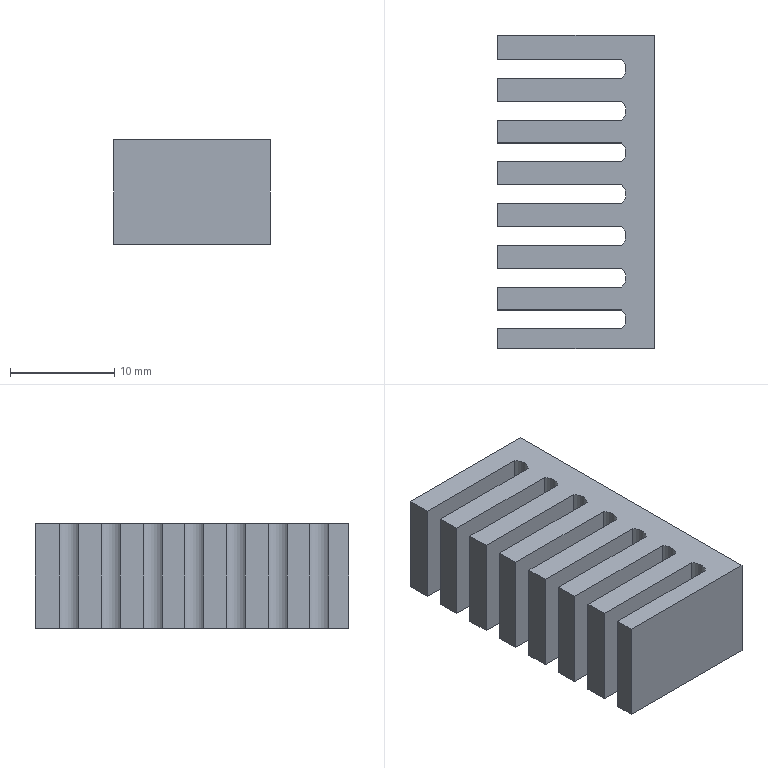Part | SolidWorks | features Extrusion 1 | 1 solid | 34 faces | box 15 x 30 x 10 mm | volume 2949 mm3 | plane 27 | cylinder 7 | commonest cylinder face diameters 2.576 x7
STEP:
#1=CARTESIAN_POINT('',(7.5,-15.,-5.));
#2=VERTEX_POINT('',#1);
#3=CARTESIAN_POINT('',(7.5,15.,-5.));
#4=VERTEX_POINT('',#3);
#5=CARTESIAN_POINT('',(7.5,-15.,-5.));
#6=DIRECTION('',(0.,1.,0.));
#7=VECTOR('',#6,1000.);
#8=LINE('',#5,#7);
#9=EDGE_CURVE('',#2,#4,#8,.T.);
#10=ORIENTED_EDGE('',*,*,#9,.T.);
#11=CARTESIAN_POINT('',(7.5,15.,5.));
#12=VERTEX_POINT('',#11);
#13=CARTESIAN_POINT('',(7.5,15.,5.));
#14=DIRECTION('',(0.,0.,-1.));
#15=VECTOR('',#14,1000.);
#16=LINE('',#13,#15);
#17=EDGE_CURVE('',#12,#4,#16,.T.);
#18=ORIENTED_EDGE('',*,*,#17,.F.);
#19=CARTESIAN_POINT('',(7.5,-15.,5.));
#20=VERTEX_POINT('',#19);
#21=CARTESIAN_POINT('',(7.5,-15.,5.));
#22=DIRECTION('',(0.,1.,0.));
#23=VECTOR('',#22,1000.);
#24=LINE('',#21,#23);
#25=EDGE_CURVE('',#20,#12,#24,.T.);
#26=ORIENTED_EDGE('',*,*,#25,.F.);
#27=CARTESIAN_POINT('',(7.5,-15.,5.));
#28=DIRECTION('',(0.,0.,-1.));
#29=VECTOR('',#28,1000.);
#30=LINE('',#27,#29);
#31=EDGE_CURVE('',#20,#2,#30,.T.);
#32=ORIENTED_EDGE('',*,*,#31,.T.);
#33=EDGE_LOOP('',(#10,#18,#26,#32));
#34=FACE_OUTER_BOUND('',#33,.T.);
#35=CARTESIAN_POINT('',(7.5,-15.,5.));
#36=DIRECTION('',(-1.,0.,0.));
#37=DIRECTION('',(0.,0.,1.));
#38=AXIS2_PLACEMENT_3D('',#35,#36,#37);
#39=PLANE('',#38);
#40=ADVANCED_FACE('',(#34),#39,.F.);
#41=CARTESIAN_POINT('',(-7.5,15.,-5.));
#42=VERTEX_POINT('',#41);
#43=CARTESIAN_POINT('',(7.5,15.,-5.));
#44=DIRECTION('',(-1.,0.,0.));
#45=VECTOR('',#44,1000.);
#46=LINE('',#43,#45);
#47=EDGE_CURVE('',#4,#42,#46,.T.);
#48=ORIENTED_EDGE('',*,*,#47,.T.);
#49=CARTESIAN_POINT('',(-7.5,15.,5.));
#50=VERTEX_POINT('',#49);
#51=CARTESIAN_POINT('',(-7.5,15.,5.));
#52=DIRECTION('',(0.,0.,-1.));
#53=VECTOR('',#52,1000.);
#54=LINE('',#51,#53);
#55=EDGE_CURVE('',#50,#42,#54,.T.);
#56=ORIENTED_EDGE('',*,*,#55,.F.);
#57=CARTESIAN_POINT('',(7.5,15.,5.));
#58=DIRECTION('',(-1.,0.,0.));
#59=VECTOR('',#58,1000.);
#60=LINE('',#57,#59);
#61=EDGE_CURVE('',#12,#50,#60,.T.);
#62=ORIENTED_EDGE('',*,*,#61,.F.);
#63=ORIENTED_EDGE('',*,*,#17,.T.);
#64=EDGE_LOOP('',(#48,#56,#62,#63));
#65=FACE_OUTER_BOUND('',#64,.T.);
#66=CARTESIAN_POINT('',(7.5,15.,5.));
#67=DIRECTION('',(0.,-1.,0.));
#68=DIRECTION('',(1.,0.,0.));
#69=AXIS2_PLACEMENT_3D('',#66,#67,#68);
#70=PLANE('',#69);
#71=ADVANCED_FACE('',(#65),#70,.F.);
#72=CARTESIAN_POINT('',(-7.5,12.696,-5.));
#73=VERTEX_POINT('',#72);
#74=CARTESIAN_POINT('',(-7.5,12.696,-5.));
#75=DIRECTION('',(0.,-1.,0.));
#76=VECTOR('',#75,1000.);
#77=LINE('',#74,#76);
#78=EDGE_CURVE('',#42,#73,#77,.T.);
#79=ORIENTED_EDGE('',*,*,#78,.T.);
#80=CARTESIAN_POINT('',(-7.5,12.696,5.));
#81=VERTEX_POINT('',#80);
#82=CARTESIAN_POINT('',(-7.5,12.696,5.));
#83=DIRECTION('',(0.,0.,-1.));
#84=VECTOR('',#83,1000.);
#85=LINE('',#82,#84);
#86=EDGE_CURVE('',#81,#73,#85,.T.);
#87=ORIENTED_EDGE('',*,*,#86,.F.);
#88=CARTESIAN_POINT('',(-7.5,12.696,5.));
#89=DIRECTION('',(0.,-1.,0.));
#90=VECTOR('',#89,1000.);
#91=LINE('',#88,#90);
#92=EDGE_CURVE('',#50,#81,#91,.T.);
#93=ORIENTED_EDGE('',*,*,#92,.F.);
#94=ORIENTED_EDGE('',*,*,#55,.T.);
#95=EDGE_LOOP('',(#79,#87,#93,#94));
#96=FACE_OUTER_BOUND('',#95,.T.);
#97=CARTESIAN_POINT('',(-7.5,12.696,5.));
#98=DIRECTION('',(1.,0.,0.));
#99=DIRECTION('',(0.,0.,-1.));
#100=AXIS2_PLACEMENT_3D('',#97,#98,#99);
#101=PLANE('',#100);
#102=ADVANCED_FACE('',(#96),#101,.F.);
#103=CARTESIAN_POINT('',(4.407,12.696,-5.));
#104=VERTEX_POINT('',#103);
#105=CARTESIAN_POINT('',(4.407,12.696,-5.));
#106=DIRECTION('',(1.,0.,0.));
#107=VECTOR('',#106,1000.);
#108=LINE('',#105,#107);
#109=EDGE_CURVE('',#73,#104,#108,.T.);
#110=ORIENTED_EDGE('',*,*,#109,.T.);
#111=CARTESIAN_POINT('',(4.407,12.696,5.));
#112=VERTEX_POINT('',#111);
#113=CARTESIAN_POINT('',(4.407,12.696,5.));
#114=DIRECTION('',(0.,0.,-1.));
#115=VECTOR('',#114,1000.);
#116=LINE('',#113,#115);
#117=EDGE_CURVE('',#112,#104,#116,.T.);
#118=ORIENTED_EDGE('',*,*,#117,.F.);
#119=CARTESIAN_POINT('',(4.407,12.696,5.));
#120=DIRECTION('',(1.,0.,0.));
#121=VECTOR('',#120,1000.);
#122=LINE('',#119,#121);
#123=EDGE_CURVE('',#81,#112,#122,.T.);
#124=ORIENTED_EDGE('',*,*,#123,.F.);
#125=ORIENTED_EDGE('',*,*,#86,.T.);
#126=EDGE_LOOP('',(#110,#118,#124,#125));
#127=FACE_OUTER_BOUND('',#126,.T.);
#128=CARTESIAN_POINT('',(4.407,12.696,5.));
#129=DIRECTION('',(0.,1.,0.));
#130=DIRECTION('',(0.,0.,1.));
#131=AXIS2_PLACEMENT_3D('',#128,#129,#130);
#132=PLANE('',#131);
#133=ADVANCED_FACE('',(#127),#132,.F.);
#134=CARTESIAN_POINT('',(4.407,10.874,-5.));
#135=VERTEX_POINT('',#134);
#136=CARTESIAN_POINT('',(3.497,11.785,-5.));
#137=DIRECTION('',(0.,0.,-1.));
#138=DIRECTION('',(1.,0.,0.));
#139=AXIS2_PLACEMENT_3D('',#136,#137,#138);
#140=CIRCLE('',#139,1.288);
#141=EDGE_CURVE('',#104,#135,#140,.T.);
#142=ORIENTED_EDGE('',*,*,#141,.T.);
#143=CARTESIAN_POINT('',(4.407,10.874,5.));
#144=VERTEX_POINT('',#143);
#145=CARTESIAN_POINT('',(4.407,10.874,5.));
#146=DIRECTION('',(0.,0.,-1.));
#147=VECTOR('',#146,1000.);
#148=LINE('',#145,#147);
#149=EDGE_CURVE('',#144,#135,#148,.T.);
#150=ORIENTED_EDGE('',*,*,#149,.F.);
#151=CARTESIAN_POINT('',(3.497,11.785,5.));
#152=DIRECTION('',(0.,0.,-1.));
#153=DIRECTION('',(1.,0.,0.));
#154=AXIS2_PLACEMENT_3D('',#151,#152,#153);
#155=CIRCLE('',#154,1.288);
#156=EDGE_CURVE('',#112,#144,#155,.T.);
#157=ORIENTED_EDGE('',*,*,#156,.F.);
#158=ORIENTED_EDGE('',*,*,#117,.T.);
#159=EDGE_LOOP('',(#142,#150,#157,#158));
#160=FACE_OUTER_BOUND('',#159,.T.);
#161=CARTESIAN_POINT('',(3.497,11.785,5.));
#162=DIRECTION('',(0.,0.,-1.));
#163=DIRECTION('',(-1.,0.,0.));
#164=AXIS2_PLACEMENT_3D('',#161,#162,#163);
#165=CYLINDRICAL_SURFACE('',#164,1.288);
#166=ADVANCED_FACE('',(#160),#165,.F.);
#167=CARTESIAN_POINT('',(-7.5,10.874,-5.));
#168=VERTEX_POINT('',#167);
#169=CARTESIAN_POINT('',(-7.5,10.874,-5.));
#170=DIRECTION('',(-1.,0.,0.));
#171=VECTOR('',#170,1000.);
#172=LINE('',#169,#171);
#173=EDGE_CURVE('',#135,#168,#172,.T.);
#174=ORIENTED_EDGE('',*,*,#173,.T.);
#175=CARTESIAN_POINT('',(-7.5,10.874,5.));
#176=VERTEX_POINT('',#175);
#177=CARTESIAN_POINT('',(-7.5,10.874,5.));
#178=DIRECTION('',(0.,0.,-1.));
#179=VECTOR('',#178,1000.);
#180=LINE('',#177,#179);
#181=EDGE_CURVE('',#176,#168,#180,.T.);
#182=ORIENTED_EDGE('',*,*,#181,.F.);
#183=CARTESIAN_POINT('',(-7.5,10.874,5.));
#184=DIRECTION('',(-1.,0.,0.));
#185=VECTOR('',#184,1000.);
#186=LINE('',#183,#185);
#187=EDGE_CURVE('',#144,#176,#186,.T.);
#188=ORIENTED_EDGE('',*,*,#187,.F.);
#189=ORIENTED_EDGE('',*,*,#149,.T.);
#190=EDGE_LOOP('',(#174,#182,#188,#189));
#191=FACE_OUTER_BOUND('',#190,.T.);
#192=CARTESIAN_POINT('',(-7.5,10.874,5.));
#193=DIRECTION('',(0.,-1.,0.));
#194=DIRECTION('',(0.,0.,-1.));
#195=AXIS2_PLACEMENT_3D('',#192,#193,#194);
#196=PLANE('',#195);
#197=ADVANCED_FACE('',(#191),#196,.F.);
#198=CARTESIAN_POINT('',(-7.5,8.696,-5.));
#199=VERTEX_POINT('',#198);
#200=CARTESIAN_POINT('',(-7.5,8.696,-5.));
#201=DIRECTION('',(0.,-1.,0.));
#202=VECTOR('',#201,1000.);
#203=LINE('',#200,#202);
#204=EDGE_CURVE('',#168,#199,#203,.T.);
#205=ORIENTED_EDGE('',*,*,#204,.T.);
#206=CARTESIAN_POINT('',(-7.5,8.696,5.));
#207=VERTEX_POINT('',#206);
#208=CARTESIAN_POINT('',(-7.5,8.696,5.));
#209=DIRECTION('',(0.,0.,-1.));
#210=VECTOR('',#209,1000.);
#211=LINE('',#208,#210);
#212=EDGE_CURVE('',#207,#199,#211,.T.);
#213=ORIENTED_EDGE('',*,*,#212,.F.);
#214=CARTESIAN_POINT('',(-7.5,8.696,5.));
#215=DIRECTION('',(0.,-1.,0.));
#216=VECTOR('',#215,1000.);
#217=LINE('',#214,#216);
#218=EDGE_CURVE('',#176,#207,#217,.T.);
#219=ORIENTED_EDGE('',*,*,#218,.F.);
#220=ORIENTED_EDGE('',*,*,#181,.T.);
#221=EDGE_LOOP('',(#205,#213,#219,#220));
#222=FACE_OUTER_BOUND('',#221,.T.);
#223=CARTESIAN_POINT('',(-7.5,8.696,5.));
#224=DIRECTION('',(1.,0.,0.));
#225=DIRECTION('',(0.,0.,-1.));
#226=AXIS2_PLACEMENT_3D('',#223,#224,#225);
#227=PLANE('',#226);
#228=ADVANCED_FACE('',(#222),#227,.F.);
#229=CARTESIAN_POINT('',(4.407,8.696,-5.));
#230=VERTEX_POINT('',#229);
#231=CARTESIAN_POINT('',(4.407,8.696,-5.));
#232=DIRECTION('',(1.,0.,0.));
#233=VECTOR('',#232,1000.);
#234=LINE('',#231,#233);
#235=EDGE_CURVE('',#199,#230,#234,.T.);
#236=ORIENTED_EDGE('',*,*,#235,.T.);
#237=CARTESIAN_POINT('',(4.407,8.696,5.));
#238=VERTEX_POINT('',#237);
#239=CARTESIAN_POINT('',(4.407,8.696,5.));
#240=DIRECTION('',(0.,0.,-1.));
#241=VECTOR('',#240,1000.);
#242=LINE('',#239,#241);
#243=EDGE_CURVE('',#238,#230,#242,.T.);
#244=ORIENTED_EDGE('',*,*,#243,.F.);
#245=CARTESIAN_POINT('',(4.407,8.696,5.));
#246=DIRECTION('',(1.,0.,0.));
#247=VECTOR('',#246,1000.);
#248=LINE('',#245,#247);
#249=EDGE_CURVE('',#207,#238,#248,.T.);
#250=ORIENTED_EDGE('',*,*,#249,.F.);
#251=ORIENTED_EDGE('',*,*,#212,.T.);
#252=EDGE_LOOP('',(#236,#244,#250,#251));
#253=FACE_OUTER_BOUND('',#252,.T.);
#254=CARTESIAN_POINT('',(4.407,8.696,5.));
#255=DIRECTION('',(0.,1.,0.));
#256=DIRECTION('',(0.,0.,1.));
#257=AXIS2_PLACEMENT_3D('',#254,#255,#256);
#258=PLANE('',#257);
#259=ADVANCED_FACE('',(#253),#258,.F.);
#260=CARTESIAN_POINT('',(4.407,6.874,-5.));
#261=VERTEX_POINT('',#260);
#262=CARTESIAN_POINT('',(3.497,7.785,-5.));
#263=DIRECTION('',(0.,0.,-1.));
#264=DIRECTION('',(1.,0.,0.));
#265=AXIS2_PLACEMENT_3D('',#262,#263,#264);
#266=CIRCLE('',#265,1.288);
#267=EDGE_CURVE('',#230,#261,#266,.T.);
#268=ORIENTED_EDGE('',*,*,#267,.T.);
#269=CARTESIAN_POINT('',(4.407,6.874,5.));
#270=VERTEX_POINT('',#269);
#271=CARTESIAN_POINT('',(4.407,6.874,5.));
#272=DIRECTION('',(0.,0.,-1.));
#273=VECTOR('',#272,1000.);
#274=LINE('',#271,#273);
#275=EDGE_CURVE('',#270,#261,#274,.T.);
#276=ORIENTED_EDGE('',*,*,#275,.F.);
#277=CARTESIAN_POINT('',(3.497,7.785,5.));
#278=DIRECTION('',(0.,0.,-1.));
#279=DIRECTION('',(1.,0.,0.));
#280=AXIS2_PLACEMENT_3D('',#277,#278,#279);
#281=CIRCLE('',#280,1.288);
#282=EDGE_CURVE('',#238,#270,#281,.T.);
#283=ORIENTED_EDGE('',*,*,#282,.F.);
#284=ORIENTED_EDGE('',*,*,#243,.T.);
#285=EDGE_LOOP('',(#268,#276,#283,#284));
#286=FACE_OUTER_BOUND('',#285,.T.);
#287=CARTESIAN_POINT('',(3.497,7.785,5.));
#288=DIRECTION('',(0.,0.,-1.));
#289=DIRECTION('',(-1.,0.,0.));
#290=AXIS2_PLACEMENT_3D('',#287,#288,#289);
#291=CYLINDRICAL_SURFACE('',#290,1.288);
#292=ADVANCED_FACE('',(#286),#291,.F.);
#293=CARTESIAN_POINT('',(-7.5,6.874,-5.));
#294=VERTEX_POINT('',#293);
#295=CARTESIAN_POINT('',(-7.5,6.874,-5.));
#296=DIRECTION('',(-1.,0.,0.));
#297=VECTOR('',#296,1000.);
#298=LINE('',#295,#297);
#299=EDGE_CURVE('',#261,#294,#298,.T.);
#300=ORIENTED_EDGE('',*,*,#299,.T.);
#301=CARTESIAN_POINT('',(-7.5,6.874,5.));
#302=VERTEX_POINT('',#301);
#303=CARTESIAN_POINT('',(-7.5,6.874,5.));
#304=DIRECTION('',(0.,0.,-1.));
#305=VECTOR('',#304,1000.);
#306=LINE('',#303,#305);
#307=EDGE_CURVE('',#302,#294,#306,.T.);
#308=ORIENTED_EDGE('',*,*,#307,.F.);
#309=CARTESIAN_POINT('',(-7.5,6.874,5.));
#310=DIRECTION('',(-1.,0.,0.));
#311=VECTOR('',#310,1000.);
#312=LINE('',#309,#311);
#313=EDGE_CURVE('',#270,#302,#312,.T.);
#314=ORIENTED_EDGE('',*,*,#313,.F.);
#315=ORIENTED_EDGE('',*,*,#275,.T.);
#316=EDGE_LOOP('',(#300,#308,#314,#315));
#317=FACE_OUTER_BOUND('',#316,.T.);
#318=CARTESIAN_POINT('',(-7.5,6.874,5.));
#319=DIRECTION('',(0.,-1.,0.));
#320=DIRECTION('',(0.,0.,-1.));
#321=AXIS2_PLACEMENT_3D('',#318,#319,#320);
#322=PLANE('',#321);
#323=ADVANCED_FACE('',(#317),#322,.F.);
#324=CARTESIAN_POINT('',(-7.5,4.696,-5.));
#325=VERTEX_POINT('',#324);
#326=CARTESIAN_POINT('',(-7.5,6.874,-5.));
#327=DIRECTION('',(0.,-1.,0.));
#328=VECTOR('',#327,1000.);
#329=LINE('',#326,#328);
#330=EDGE_CURVE('',#294,#325,#329,.T.);
#331=ORIENTED_EDGE('',*,*,#330,.T.);
#332=CARTESIAN_POINT('',(-7.5,4.696,5.));
#333=VERTEX_POINT('',#332);
#334=CARTESIAN_POINT('',(-7.5,4.696,5.));
#335=DIRECTION('',(0.,0.,-1.));
#336=VECTOR('',#335,1000.);
#337=LINE('',#334,#336);
#338=EDGE_CURVE('',#333,#325,#337,.T.);
#339=ORIENTED_EDGE('',*,*,#338,.F.);
#340=CARTESIAN_POINT('',(-7.5,6.874,5.));
#341=DIRECTION('',(0.,-1.,0.));
#342=VECTOR('',#341,1000.);
#343=LINE('',#340,#342);
#344=EDGE_CURVE('',#302,#333,#343,.T.);
#345=ORIENTED_EDGE('',*,*,#344,.F.);
#346=ORIENTED_EDGE('',*,*,#307,.T.);
#347=EDGE_LOOP('',(#331,#339,#345,#346));
#348=FACE_OUTER_BOUND('',#347,.T.);
#349=CARTESIAN_POINT('',(-7.5,6.874,5.));
#350=DIRECTION('',(1.,0.,0.));
#351=DIRECTION('',(0.,0.,-1.));
#352=AXIS2_PLACEMENT_3D('',#349,#350,#351);
#353=PLANE('',#352);
#354=ADVANCED_FACE('',(#348),#353,.F.);
#355=CARTESIAN_POINT('',(4.407,4.696,-5.));
#356=VERTEX_POINT('',#355);
#357=CARTESIAN_POINT('',(4.407,4.696,-5.));
#358=DIRECTION('',(1.,0.,0.));
#359=VECTOR('',#358,1000.);
#360=LINE('',#357,#359);
#361=EDGE_CURVE('',#325,#356,#360,.T.);
#362=ORIENTED_EDGE('',*,*,#361,.T.);
#363=CARTESIAN_POINT('',(4.407,4.696,5.));
#364=VERTEX_POINT('',#363);
#365=CARTESIAN_POINT('',(4.407,4.696,5.));
#366=DIRECTION('',(0.,0.,-1.));
#367=VECTOR('',#366,1000.);
#368=LINE('',#365,#367);
#369=EDGE_CURVE('',#364,#356,#368,.T.);
#370=ORIENTED_EDGE('',*,*,#369,.F.);
#371=CARTESIAN_POINT('',(4.407,4.696,5.));
#372=DIRECTION('',(1.,0.,0.));
#373=VECTOR('',#372,1000.);
#374=LINE('',#371,#373);
#375=EDGE_CURVE('',#333,#364,#374,.T.);
#376=ORIENTED_EDGE('',*,*,#375,.F.);
#377=ORIENTED_EDGE('',*,*,#338,.T.);
#378=EDGE_LOOP('',(#362,#370,#376,#377));
#379=FACE_OUTER_BOUND('',#378,.T.);
#380=CARTESIAN_POINT('',(4.407,4.696,5.));
#381=DIRECTION('',(0.,1.,0.));
#382=DIRECTION('',(0.,0.,1.));
#383=AXIS2_PLACEMENT_3D('',#380,#381,#382);
#384=PLANE('',#383);
#385=ADVANCED_FACE('',(#379),#384,.F.);
#386=CARTESIAN_POINT('',(4.407,2.874,-5.));
#387=VERTEX_POINT('',#386);
#388=CARTESIAN_POINT('',(3.497,3.785,-5.));
#389=DIRECTION('',(0.,0.,-1.));
#390=DIRECTION('',(1.,0.,0.));
#391=AXIS2_PLACEMENT_3D('',#388,#389,#390);
#392=CIRCLE('',#391,1.288);
#393=EDGE_CURVE('',#356,#387,#392,.T.);
#394=ORIENTED_EDGE('',*,*,#393,.T.);
#395=CARTESIAN_POINT('',(4.407,2.874,5.));
#396=VERTEX_POINT('',#395);
#397=CARTESIAN_POINT('',(4.407,2.874,5.));
#398=DIRECTION('',(0.,0.,-1.));
#399=VECTOR('',#398,1000.);
#400=LINE('',#397,#399);
#401=EDGE_CURVE('',#396,#387,#400,.T.);
#402=ORIENTED_EDGE('',*,*,#401,.F.);
#403=CARTESIAN_POINT('',(3.497,3.785,5.));
#404=DIRECTION('',(0.,0.,-1.));
#405=DIRECTION('',(1.,0.,0.));
#406=AXIS2_PLACEMENT_3D('',#403,#404,#405);
#407=CIRCLE('',#406,1.288);
#408=EDGE_CURVE('',#364,#396,#407,.T.);
#409=ORIENTED_EDGE('',*,*,#408,.F.);
#410=ORIENTED_EDGE('',*,*,#369,.T.);
#411=EDGE_LOOP('',(#394,#402,#409,#410));
#412=FACE_OUTER_BOUND('',#411,.T.);
#413=CARTESIAN_POINT('',(3.497,3.785,5.));
#414=DIRECTION('',(0.,0.,-1.));
#415=DIRECTION('',(-1.,0.,0.));
#416=AXIS2_PLACEMENT_3D('',#413,#414,#415);
#417=CYLINDRICAL_SURFACE('',#416,1.288);
#418=ADVANCED_FACE('',(#412),#417,.F.);
#419=CARTESIAN_POINT('',(-7.5,2.874,-5.));
#420=VERTEX_POINT('',#419);
#421=CARTESIAN_POINT('',(-7.5,2.874,-5.));
#422=DIRECTION('',(-1.,0.,0.));
#423=VECTOR('',#422,1000.);
#424=LINE('',#421,#423);
#425=EDGE_CURVE('',#387,#420,#424,.T.);
#426=ORIENTED_EDGE('',*,*,#425,.T.);
#427=CARTESIAN_POINT('',(-7.5,2.874,5.));
#428=VERTEX_POINT('',#427);
#429=CARTESIAN_POINT('',(-7.5,2.874,5.));
#430=DIRECTION('',(0.,0.,-1.));
#431=VECTOR('',#430,1000.);
#432=LINE('',#429,#431);
#433=EDGE_CURVE('',#428,#420,#432,.T.);
#434=ORIENTED_EDGE('',*,*,#433,.F.);
#435=CARTESIAN_POINT('',(-7.5,2.874,5.));
#436=DIRECTION('',(-1.,0.,0.));
#437=VECTOR('',#436,1000.);
#438=LINE('',#435,#437);
#439=EDGE_CURVE('',#396,#428,#438,.T.);
#440=ORIENTED_EDGE('',*,*,#439,.F.);
#441=ORIENTED_EDGE('',*,*,#401,.T.);
#442=EDGE_LOOP('',(#426,#434,#440,#441));
#443=FACE_OUTER_BOUND('',#442,.T.);
#444=CARTESIAN_POINT('',(-7.5,2.874,5.));
#445=DIRECTION('',(0.,-1.,0.));
#446=DIRECTION('',(0.,0.,-1.));
#447=AXIS2_PLACEMENT_3D('',#444,#445,#446);
#448=PLANE('',#447);
#449=ADVANCED_FACE('',(#443),#448,.F.);
#450=CARTESIAN_POINT('',(-7.5,0.6956,-5.));
#451=VERTEX_POINT('',#450);
#452=CARTESIAN_POINT('',(-7.5,0.6956,-5.));
#453=DIRECTION('',(0.,-1.,0.));
#454=VECTOR('',#453,1000.);
#455=LINE('',#452,#454);
#456=EDGE_CURVE('',#420,#451,#455,.T.);
#457=ORIENTED_EDGE('',*,*,#456,.T.);
#458=CARTESIAN_POINT('',(-7.5,0.6956,5.));
#459=VERTEX_POINT('',#458);
#460=CARTESIAN_POINT('',(-7.5,0.6956,5.));
#461=DIRECTION('',(0.,0.,-1.));
#462=VECTOR('',#461,1000.);
#463=LINE('',#460,#462);
#464=EDGE_CURVE('',#459,#451,#463,.T.);
#465=ORIENTED_EDGE('',*,*,#464,.F.);
#466=CARTESIAN_POINT('',(-7.5,0.6956,5.));
#467=DIRECTION('',(0.,-1.,0.));
#468=VECTOR('',#467,1000.);
#469=LINE('',#466,#468);
#470=EDGE_CURVE('',#428,#459,#469,.T.);
#471=ORIENTED_EDGE('',*,*,#470,.F.);
#472=ORIENTED_EDGE('',*,*,#433,.T.);
#473=EDGE_LOOP('',(#457,#465,#471,#472));
#474=FACE_OUTER_BOUND('',#473,.T.);
#475=CARTESIAN_POINT('',(-7.5,0.6956,5.));
#476=DIRECTION('',(1.,0.,0.));
#477=DIRECTION('',(0.,0.,-1.));
#478=AXIS2_PLACEMENT_3D('',#475,#476,#477);
#479=PLANE('',#478);
#480=ADVANCED_FACE('',(#474),#479,.F.);
#481=CARTESIAN_POINT('',(4.407,0.6956,-5.));
#482=VERTEX_POINT('',#481);
#483=CARTESIAN_POINT('',(4.407,0.6956,-5.));
#484=DIRECTION('',(1.,0.,0.));
#485=VECTOR('',#484,1000.);
#486=LINE('',#483,#485);
#487=EDGE_CURVE('',#451,#482,#486,.T.);
#488=ORIENTED_EDGE('',*,*,#487,.T.);
#489=CARTESIAN_POINT('',(4.407,0.6956,5.));
#490=VERTEX_POINT('',#489);
#491=CARTESIAN_POINT('',(4.407,0.6956,5.));
#492=DIRECTION('',(0.,0.,-1.));
#493=VECTOR('',#492,1000.);
#494=LINE('',#491,#493);
#495=EDGE_CURVE('',#490,#482,#494,.T.);
#496=ORIENTED_EDGE('',*,*,#495,.F.);
#497=CARTESIAN_POINT('',(4.407,0.6956,5.));
#498=DIRECTION('',(1.,0.,0.));
#499=VECTOR('',#498,1000.);
#500=LINE('',#497,#499);
#501=EDGE_CURVE('',#459,#490,#500,.T.);
#502=ORIENTED_EDGE('',*,*,#501,.F.);
#503=ORIENTED_EDGE('',*,*,#464,.T.);
#504=EDGE_LOOP('',(#488,#496,#502,#503));
#505=FACE_OUTER_BOUND('',#504,.T.);
#506=CARTESIAN_POINT('',(4.407,0.6956,5.));
#507=DIRECTION('',(0.,1.,0.));
#508=DIRECTION('',(0.,0.,1.));
#509=AXIS2_PLACEMENT_3D('',#506,#507,#508);
#510=PLANE('',#509);
#511=ADVANCED_FACE('',(#505),#510,.F.);
#512=CARTESIAN_POINT('',(4.407,-1.126,-5.));
#513=VERTEX_POINT('',#512);
#514=CARTESIAN_POINT('',(3.497,-0.2151,-5.));
#515=DIRECTION('',(0.,0.,-1.));
#516=DIRECTION('',(1.,0.,0.));
#517=AXIS2_PLACEMENT_3D('',#514,#515,#516);
#518=CIRCLE('',#517,1.288);
#519=EDGE_CURVE('',#482,#513,#518,.T.);
#520=ORIENTED_EDGE('',*,*,#519,.T.);
#521=CARTESIAN_POINT('',(4.407,-1.126,5.));
#522=VERTEX_POINT('',#521);
#523=CARTESIAN_POINT('',(4.407,-1.126,5.));
#524=DIRECTION('',(0.,0.,-1.));
#525=VECTOR('',#524,1000.);
#526=LINE('',#523,#525);
#527=EDGE_CURVE('',#522,#513,#526,.T.);
#528=ORIENTED_EDGE('',*,*,#527,.F.);
#529=CARTESIAN_POINT('',(3.497,-0.2151,5.));
#530=DIRECTION('',(0.,0.,-1.));
#531=DIRECTION('',(1.,0.,0.));
#532=AXIS2_PLACEMENT_3D('',#529,#530,#531);
#533=CIRCLE('',#532,1.288);
#534=EDGE_CURVE('',#490,#522,#533,.T.);
#535=ORIENTED_EDGE('',*,*,#534,.F.);
#536=ORIENTED_EDGE('',*,*,#495,.T.);
#537=EDGE_LOOP('',(#520,#528,#535,#536));
#538=FACE_OUTER_BOUND('',#537,.T.);
#539=CARTESIAN_POINT('',(3.497,-0.2151,5.));
#540=DIRECTION('',(0.,0.,-1.));
#541=DIRECTION('',(-1.,0.,0.));
#542=AXIS2_PLACEMENT_3D('',#539,#540,#541);
#543=CYLINDRICAL_SURFACE('',#542,1.288);
#544=ADVANCED_FACE('',(#538),#543,.F.);
#545=CARTESIAN_POINT('',(-7.5,-1.126,-5.));
#546=VERTEX_POINT('',#545);
#547=CARTESIAN_POINT('',(-7.5,-1.126,-5.));
#548=DIRECTION('',(-1.,0.,0.));
#549=VECTOR('',#548,1000.);
#550=LINE('',#547,#549);
#551=EDGE_CURVE('',#513,#546,#550,.T.);
#552=ORIENTED_EDGE('',*,*,#551,.T.);
#553=CARTESIAN_POINT('',(-7.5,-1.126,5.));
#554=VERTEX_POINT('',#553);
#555=CARTESIAN_POINT('',(-7.5,-1.126,5.));
#556=DIRECTION('',(0.,0.,-1.));
#557=VECTOR('',#556,1000.);
#558=LINE('',#555,#557);
#559=EDGE_CURVE('',#554,#546,#558,.T.);
#560=ORIENTED_EDGE('',*,*,#559,.F.);
#561=CARTESIAN_POINT('',(-7.5,-1.126,5.));
#562=DIRECTION('',(-1.,0.,0.));
#563=VECTOR('',#562,1000.);
#564=LINE('',#561,#563);
#565=EDGE_CURVE('',#522,#554,#564,.T.);
#566=ORIENTED_EDGE('',*,*,#565,.F.);
#567=ORIENTED_EDGE('',*,*,#527,.T.);
#568=EDGE_LOOP('',(#552,#560,#566,#567));
#569=FACE_OUTER_BOUND('',#568,.T.);
#570=CARTESIAN_POINT('',(-7.5,-1.126,5.));
#571=DIRECTION('',(0.,-1.,0.));
#572=DIRECTION('',(0.,0.,-1.));
#573=AXIS2_PLACEMENT_3D('',#570,#571,#572);
#574=PLANE('',#573);
#575=ADVANCED_FACE('',(#569),#574,.F.);
#576=CARTESIAN_POINT('',(-7.5,-3.304,-5.));
#577=VERTEX_POINT('',#576);
#578=CARTESIAN_POINT('',(-7.5,-3.304,-5.));
#579=DIRECTION('',(0.,-1.,0.));
#580=VECTOR('',#579,1000.);
#581=LINE('',#578,#580);
#582=EDGE_CURVE('',#546,#577,#581,.T.);
#583=ORIENTED_EDGE('',*,*,#582,.T.);
#584=CARTESIAN_POINT('',(-7.5,-3.304,5.));
#585=VERTEX_POINT('',#584);
#586=CARTESIAN_POINT('',(-7.5,-3.304,5.));
#587=DIRECTION('',(0.,0.,-1.));
#588=VECTOR('',#587,1000.);
#589=LINE('',#586,#588);
#590=EDGE_CURVE('',#585,#577,#589,.T.);
#591=ORIENTED_EDGE('',*,*,#590,.F.);
#592=CARTESIAN_POINT('',(-7.5,-3.304,5.));
#593=DIRECTION('',(0.,-1.,0.));
#594=VECTOR('',#593,1000.);
#595=LINE('',#592,#594);
#596=EDGE_CURVE('',#554,#585,#595,.T.);
#597=ORIENTED_EDGE('',*,*,#596,.F.);
#598=ORIENTED_EDGE('',*,*,#559,.T.);
#599=EDGE_LOOP('',(#583,#591,#597,#598));
#600=FACE_OUTER_BOUND('',#599,.T.);
#601=CARTESIAN_POINT('',(-7.5,-3.304,5.));
#602=DIRECTION('',(1.,0.,0.));
#603=DIRECTION('',(0.,0.,-1.));
#604=AXIS2_PLACEMENT_3D('',#601,#602,#603);
#605=PLANE('',#604);
#606=ADVANCED_FACE('',(#600),#605,.F.);
#607=CARTESIAN_POINT('',(4.407,-3.304,-5.));
#608=VERTEX_POINT('',#607);
#609=CARTESIAN_POINT('',(4.407,-3.304,-5.));
#610=DIRECTION('',(1.,0.,0.));
#611=VECTOR('',#610,1000.);
#612=LINE('',#609,#611);
#613=EDGE_CURVE('',#577,#608,#612,.T.);
#614=ORIENTED_EDGE('',*,*,#613,.T.);
#615=CARTESIAN_POINT('',(4.407,-3.304,5.));
#616=VERTEX_POINT('',#615);
#617=CARTESIAN_POINT('',(4.407,-3.304,5.));
#618=DIRECTION('',(0.,0.,-1.));
#619=VECTOR('',#618,1000.);
#620=LINE('',#617,#619);
#621=EDGE_CURVE('',#616,#608,#620,.T.);
#622=ORIENTED_EDGE('',*,*,#621,.F.);
#623=CARTESIAN_POINT('',(4.407,-3.304,5.));
#624=DIRECTION('',(1.,0.,0.));
#625=VECTOR('',#624,1000.);
#626=LINE('',#623,#625);
#627=EDGE_CURVE('',#585,#616,#626,.T.);
#628=ORIENTED_EDGE('',*,*,#627,.F.);
#629=ORIENTED_EDGE('',*,*,#590,.T.);
#630=EDGE_LOOP('',(#614,#622,#628,#629));
#631=FACE_OUTER_BOUND('',#630,.T.);
#632=CARTESIAN_POINT('',(4.407,-3.304,5.));
#633=DIRECTION('',(0.,1.,0.));
#634=DIRECTION('',(0.,0.,1.));
#635=AXIS2_PLACEMENT_3D('',#632,#633,#634);
#636=PLANE('',#635);
#637=ADVANCED_FACE('',(#631),#636,.F.);
#638=CARTESIAN_POINT('',(4.407,-5.126,-5.));
#639=VERTEX_POINT('',#638);
#640=CARTESIAN_POINT('',(3.497,-4.215,-5.));
#641=DIRECTION('',(0.,0.,-1.));
#642=DIRECTION('',(1.,0.,0.));
#643=AXIS2_PLACEMENT_3D('',#640,#641,#642);
#644=CIRCLE('',#643,1.288);
#645=EDGE_CURVE('',#608,#639,#644,.T.);
#646=ORIENTED_EDGE('',*,*,#645,.T.);
#647=CARTESIAN_POINT('',(4.407,-5.126,5.));
#648=VERTEX_POINT('',#647);
#649=CARTESIAN_POINT('',(4.407,-5.126,5.));
#650=DIRECTION('',(0.,0.,-1.));
#651=VECTOR('',#650,1000.);
#652=LINE('',#649,#651);
#653=EDGE_CURVE('',#648,#639,#652,.T.);
#654=ORIENTED_EDGE('',*,*,#653,.F.);
#655=CARTESIAN_POINT('',(3.497,-4.215,5.));
#656=DIRECTION('',(0.,0.,-1.));
#657=DIRECTION('',(1.,0.,0.));
#658=AXIS2_PLACEMENT_3D('',#655,#656,#657);
#659=CIRCLE('',#658,1.288);
#660=EDGE_CURVE('',#616,#648,#659,.T.);
#661=ORIENTED_EDGE('',*,*,#660,.F.);
#662=ORIENTED_EDGE('',*,*,#621,.T.);
#663=EDGE_LOOP('',(#646,#654,#661,#662));
#664=FACE_OUTER_BOUND('',#663,.T.);
#665=CARTESIAN_POINT('',(3.497,-4.215,5.));
#666=DIRECTION('',(0.,0.,-1.));
#667=DIRECTION('',(-1.,0.,0.));
#668=AXIS2_PLACEMENT_3D('',#665,#666,#667);
#669=CYLINDRICAL_SURFACE('',#668,1.288);
#670=ADVANCED_FACE('',(#664),#669,.F.);
#671=CARTESIAN_POINT('',(-7.5,-5.126,-5.));
#672=VERTEX_POINT('',#671);
#673=CARTESIAN_POINT('',(-7.5,-5.126,-5.));
#674=DIRECTION('',(-1.,0.,0.));
#675=VECTOR('',#674,1000.);
#676=LINE('',#673,#675);
#677=EDGE_CURVE('',#639,#672,#676,.T.);
#678=ORIENTED_EDGE('',*,*,#677,.T.);
#679=CARTESIAN_POINT('',(-7.5,-5.126,5.));
#680=VERTEX_POINT('',#679);
#681=CARTESIAN_POINT('',(-7.5,-5.126,5.));
#682=DIRECTION('',(0.,0.,-1.));
#683=VECTOR('',#682,1000.);
#684=LINE('',#681,#683);
#685=EDGE_CURVE('',#680,#672,#684,.T.);
#686=ORIENTED_EDGE('',*,*,#685,.F.);
#687=CARTESIAN_POINT('',(-7.5,-5.126,5.));
#688=DIRECTION('',(-1.,0.,0.));
#689=VECTOR('',#688,1000.);
#690=LINE('',#687,#689);
#691=EDGE_CURVE('',#648,#680,#690,.T.);
#692=ORIENTED_EDGE('',*,*,#691,.F.);
#693=ORIENTED_EDGE('',*,*,#653,.T.);
#694=EDGE_LOOP('',(#678,#686,#692,#693));
#695=FACE_OUTER_BOUND('',#694,.T.);
#696=CARTESIAN_POINT('',(-7.5,-5.126,5.));
#697=DIRECTION('',(0.,-1.,0.));
#698=DIRECTION('',(0.,0.,-1.));
#699=AXIS2_PLACEMENT_3D('',#696,#697,#698);
#700=PLANE('',#699);
#701=ADVANCED_FACE('',(#695),#700,.F.);
#702=CARTESIAN_POINT('',(-7.5,-7.304,-5.));
#703=VERTEX_POINT('',#702);
#704=CARTESIAN_POINT('',(-7.5,-7.304,-5.));
#705=DIRECTION('',(0.,-1.,0.));
#706=VECTOR('',#705,1000.);
#707=LINE('',#704,#706);
#708=EDGE_CURVE('',#672,#703,#707,.T.);
#709=ORIENTED_EDGE('',*,*,#708,.T.);
#710=CARTESIAN_POINT('',(-7.5,-7.304,5.));
#711=VERTEX_POINT('',#710);
#712=CARTESIAN_POINT('',(-7.5,-7.304,5.));
#713=DIRECTION('',(0.,0.,-1.));
#714=VECTOR('',#713,1000.);
#715=LINE('',#712,#714);
#716=EDGE_CURVE('',#711,#703,#715,.T.);
#717=ORIENTED_EDGE('',*,*,#716,.F.);
#718=CARTESIAN_POINT('',(-7.5,-7.304,5.));
#719=DIRECTION('',(0.,-1.,0.));
#720=VECTOR('',#719,1000.);
#721=LINE('',#718,#720);
#722=EDGE_CURVE('',#680,#711,#721,.T.);
#723=ORIENTED_EDGE('',*,*,#722,.F.);
#724=ORIENTED_EDGE('',*,*,#685,.T.);
#725=EDGE_LOOP('',(#709,#717,#723,#724));
#726=FACE_OUTER_BOUND('',#725,.T.);
#727=CARTESIAN_POINT('',(-7.5,-7.304,5.));
#728=DIRECTION('',(1.,0.,0.));
#729=DIRECTION('',(0.,0.,-1.));
#730=AXIS2_PLACEMENT_3D('',#727,#728,#729);
#731=PLANE('',#730);
#732=ADVANCED_FACE('',(#726),#731,.F.);
#733=CARTESIAN_POINT('',(4.407,-7.304,-5.));
#734=VERTEX_POINT('',#733);
#735=CARTESIAN_POINT('',(4.407,-7.304,-5.));
#736=DIRECTION('',(1.,0.,0.));
#737=VECTOR('',#736,1000.);
#738=LINE('',#735,#737);
#739=EDGE_CURVE('',#703,#734,#738,.T.);
#740=ORIENTED_EDGE('',*,*,#739,.T.);
#741=CARTESIAN_POINT('',(4.407,-7.304,5.));
#742=VERTEX_POINT('',#741);
#743=CARTESIAN_POINT('',(4.407,-7.304,5.));
#744=DIRECTION('',(0.,0.,-1.));
#745=VECTOR('',#744,1000.);
#746=LINE('',#743,#745);
#747=EDGE_CURVE('',#742,#734,#746,.T.);
#748=ORIENTED_EDGE('',*,*,#747,.F.);
#749=CARTESIAN_POINT('',(4.407,-7.304,5.));
#750=DIRECTION('',(1.,0.,0.));
#751=VECTOR('',#750,1000.);
#752=LINE('',#749,#751);
#753=EDGE_CURVE('',#711,#742,#752,.T.);
#754=ORIENTED_EDGE('',*,*,#753,.F.);
#755=ORIENTED_EDGE('',*,*,#716,.T.);
#756=EDGE_LOOP('',(#740,#748,#754,#755));
#757=FACE_OUTER_BOUND('',#756,.T.);
#758=CARTESIAN_POINT('',(4.407,-7.304,5.));
#759=DIRECTION('',(0.,1.,0.));
#760=DIRECTION('',(0.,0.,1.));
#761=AXIS2_PLACEMENT_3D('',#758,#759,#760);
#762=PLANE('',#761);
#763=ADVANCED_FACE('',(#757),#762,.F.);
#764=CARTESIAN_POINT('',(4.407,-9.126,-5.));
#765=VERTEX_POINT('',#764);
#766=CARTESIAN_POINT('',(3.497,-8.215,-5.));
#767=DIRECTION('',(0.,0.,-1.));
#768=DIRECTION('',(1.,0.,0.));
#769=AXIS2_PLACEMENT_3D('',#766,#767,#768);
#770=CIRCLE('',#769,1.288);
#771=EDGE_CURVE('',#734,#765,#770,.T.);
#772=ORIENTED_EDGE('',*,*,#771,.T.);
#773=CARTESIAN_POINT('',(4.407,-9.126,5.));
#774=VERTEX_POINT('',#773);
#775=CARTESIAN_POINT('',(4.407,-9.126,5.));
#776=DIRECTION('',(0.,0.,-1.));
#777=VECTOR('',#776,1000.);
#778=LINE('',#775,#777);
#779=EDGE_CURVE('',#774,#765,#778,.T.);
#780=ORIENTED_EDGE('',*,*,#779,.F.);
#781=CARTESIAN_POINT('',(3.497,-8.215,5.));
#782=DIRECTION('',(0.,0.,-1.));
#783=DIRECTION('',(1.,0.,0.));
#784=AXIS2_PLACEMENT_3D('',#781,#782,#783);
#785=CIRCLE('',#784,1.288);
#786=EDGE_CURVE('',#742,#774,#785,.T.);
#787=ORIENTED_EDGE('',*,*,#786,.F.);
#788=ORIENTED_EDGE('',*,*,#747,.T.);
#789=EDGE_LOOP('',(#772,#780,#787,#788));
#790=FACE_OUTER_BOUND('',#789,.T.);
#791=CARTESIAN_POINT('',(3.497,-8.215,5.));
#792=DIRECTION('',(0.,0.,-1.));
#793=DIRECTION('',(-1.,0.,0.));
#794=AXIS2_PLACEMENT_3D('',#791,#792,#793);
#795=CYLINDRICAL_SURFACE('',#794,1.288);
#796=ADVANCED_FACE('',(#790),#795,.F.);
#797=CARTESIAN_POINT('',(-7.5,-9.126,-5.));
#798=VERTEX_POINT('',#797);
#799=CARTESIAN_POINT('',(-7.5,-9.126,-5.));
#800=DIRECTION('',(-1.,0.,0.));
#801=VECTOR('',#800,1000.);
#802=LINE('',#799,#801);
#803=EDGE_CURVE('',#765,#798,#802,.T.);
#804=ORIENTED_EDGE('',*,*,#803,.T.);
#805=CARTESIAN_POINT('',(-7.5,-9.126,5.));
#806=VERTEX_POINT('',#805);
#807=CARTESIAN_POINT('',(-7.5,-9.126,5.));
#808=DIRECTION('',(0.,0.,-1.));
#809=VECTOR('',#808,1000.);
#810=LINE('',#807,#809);
#811=EDGE_CURVE('',#806,#798,#810,.T.);
#812=ORIENTED_EDGE('',*,*,#811,.F.);
#813=CARTESIAN_POINT('',(-7.5,-9.126,5.));
#814=DIRECTION('',(-1.,0.,0.));
#815=VECTOR('',#814,1000.);
#816=LINE('',#813,#815);
#817=EDGE_CURVE('',#774,#806,#816,.T.);
#818=ORIENTED_EDGE('',*,*,#817,.F.);
#819=ORIENTED_EDGE('',*,*,#779,.T.);
#820=EDGE_LOOP('',(#804,#812,#818,#819));
#821=FACE_OUTER_BOUND('',#820,.T.);
#822=CARTESIAN_POINT('',(-7.5,-9.126,5.));
#823=DIRECTION('',(0.,-1.,0.));
#824=DIRECTION('',(0.,0.,-1.));
#825=AXIS2_PLACEMENT_3D('',#822,#823,#824);
#826=PLANE('',#825);
#827=ADVANCED_FACE('',(#821),#826,.F.);
#828=CARTESIAN_POINT('',(-7.5,-11.304,-5.));
#829=VERTEX_POINT('',#828);
#830=CARTESIAN_POINT('',(-7.5,-11.304,-5.));
#831=DIRECTION('',(0.,-1.,0.));
#832=VECTOR('',#831,1000.);
#833=LINE('',#830,#832);
#834=EDGE_CURVE('',#798,#829,#833,.T.);
#835=ORIENTED_EDGE('',*,*,#834,.T.);
#836=CARTESIAN_POINT('',(-7.5,-11.304,5.));
#837=VERTEX_POINT('',#836);
#838=CARTESIAN_POINT('',(-7.5,-11.304,5.));
#839=DIRECTION('',(0.,0.,-1.));
#840=VECTOR('',#839,1000.);
#841=LINE('',#838,#840);
#842=EDGE_CURVE('',#837,#829,#841,.T.);
#843=ORIENTED_EDGE('',*,*,#842,.F.);
#844=CARTESIAN_POINT('',(-7.5,-11.304,5.));
#845=DIRECTION('',(0.,-1.,0.));
#846=VECTOR('',#845,1000.);
#847=LINE('',#844,#846);
#848=EDGE_CURVE('',#806,#837,#847,.T.);
#849=ORIENTED_EDGE('',*,*,#848,.F.);
#850=ORIENTED_EDGE('',*,*,#811,.T.);
#851=EDGE_LOOP('',(#835,#843,#849,#850));
#852=FACE_OUTER_BOUND('',#851,.T.);
#853=CARTESIAN_POINT('',(-7.5,-11.304,5.));
#854=DIRECTION('',(1.,0.,0.));
#855=DIRECTION('',(0.,0.,-1.));
#856=AXIS2_PLACEMENT_3D('',#853,#854,#855);
#857=PLANE('',#856);
#858=ADVANCED_FACE('',(#852),#857,.F.);
#859=CARTESIAN_POINT('',(4.407,-11.304,-5.));
#860=VERTEX_POINT('',#859);
#861=CARTESIAN_POINT('',(4.407,-11.304,-5.));
#862=DIRECTION('',(1.,0.,0.));
#863=VECTOR('',#862,1000.);
#864=LINE('',#861,#863);
#865=EDGE_CURVE('',#829,#860,#864,.T.);
#866=ORIENTED_EDGE('',*,*,#865,.T.);
#867=CARTESIAN_POINT('',(4.407,-11.304,5.));
#868=VERTEX_POINT('',#867);
#869=CARTESIAN_POINT('',(4.407,-11.304,5.));
#870=DIRECTION('',(0.,0.,-1.));
#871=VECTOR('',#870,1000.);
#872=LINE('',#869,#871);
#873=EDGE_CURVE('',#868,#860,#872,.T.);
#874=ORIENTED_EDGE('',*,*,#873,.F.);
#875=CARTESIAN_POINT('',(4.407,-11.304,5.));
#876=DIRECTION('',(1.,0.,0.));
#877=VECTOR('',#876,1000.);
#878=LINE('',#875,#877);
#879=EDGE_CURVE('',#837,#868,#878,.T.);
#880=ORIENTED_EDGE('',*,*,#879,.F.);
#881=ORIENTED_EDGE('',*,*,#842,.T.);
#882=EDGE_LOOP('',(#866,#874,#880,#881));
#883=FACE_OUTER_BOUND('',#882,.T.);
#884=CARTESIAN_POINT('',(4.407,-11.304,5.));
#885=DIRECTION('',(0.,1.,0.));
#886=DIRECTION('',(0.,0.,1.));
#887=AXIS2_PLACEMENT_3D('',#884,#885,#886);
#888=PLANE('',#887);
#889=ADVANCED_FACE('',(#883),#888,.F.);
#890=CARTESIAN_POINT('',(4.407,-13.126,-5.));
#891=VERTEX_POINT('',#890);
#892=CARTESIAN_POINT('',(3.497,-12.215,-5.));
#893=DIRECTION('',(0.,0.,-1.));
#894=DIRECTION('',(1.,0.,0.));
#895=AXIS2_PLACEMENT_3D('',#892,#893,#894);
#896=CIRCLE('',#895,1.288);
#897=EDGE_CURVE('',#860,#891,#896,.T.);
#898=ORIENTED_EDGE('',*,*,#897,.T.);
#899=CARTESIAN_POINT('',(4.407,-13.126,5.));
#900=VERTEX_POINT('',#899);
#901=CARTESIAN_POINT('',(4.407,-13.126,5.));
#902=DIRECTION('',(0.,0.,-1.));
#903=VECTOR('',#902,1000.);
#904=LINE('',#901,#903);
#905=EDGE_CURVE('',#900,#891,#904,.T.);
#906=ORIENTED_EDGE('',*,*,#905,.F.);
#907=CARTESIAN_POINT('',(3.497,-12.215,5.));
#908=DIRECTION('',(0.,0.,-1.));
#909=DIRECTION('',(1.,0.,0.));
#910=AXIS2_PLACEMENT_3D('',#907,#908,#909);
#911=CIRCLE('',#910,1.288);
#912=EDGE_CURVE('',#868,#900,#911,.T.);
#913=ORIENTED_EDGE('',*,*,#912,.F.);
#914=ORIENTED_EDGE('',*,*,#873,.T.);
#915=EDGE_LOOP('',(#898,#906,#913,#914));
#916=FACE_OUTER_BOUND('',#915,.T.);
#917=CARTESIAN_POINT('',(3.497,-12.215,5.));
#918=DIRECTION('',(0.,0.,-1.));
#919=DIRECTION('',(-1.,0.,0.));
#920=AXIS2_PLACEMENT_3D('',#917,#918,#919);
#921=CYLINDRICAL_SURFACE('',#920,1.288);
#922=ADVANCED_FACE('',(#916),#921,.F.);
#923=CARTESIAN_POINT('',(-7.5,-13.126,-5.));
#924=VERTEX_POINT('',#923);
#925=CARTESIAN_POINT('',(-7.5,-13.126,-5.));
#926=DIRECTION('',(-1.,0.,0.));
#927=VECTOR('',#926,1000.);
#928=LINE('',#925,#927);
#929=EDGE_CURVE('',#891,#924,#928,.T.);
#930=ORIENTED_EDGE('',*,*,#929,.T.);
#931=CARTESIAN_POINT('',(-7.5,-13.126,5.));
#932=VERTEX_POINT('',#931);
#933=CARTESIAN_POINT('',(-7.5,-13.126,5.));
#934=DIRECTION('',(0.,0.,-1.));
#935=VECTOR('',#934,1000.);
#936=LINE('',#933,#935);
#937=EDGE_CURVE('',#932,#924,#936,.T.);
#938=ORIENTED_EDGE('',*,*,#937,.F.);
#939=CARTESIAN_POINT('',(-7.5,-13.126,5.));
#940=DIRECTION('',(-1.,0.,0.));
#941=VECTOR('',#940,1000.);
#942=LINE('',#939,#941);
#943=EDGE_CURVE('',#900,#932,#942,.T.);
#944=ORIENTED_EDGE('',*,*,#943,.F.);
#945=ORIENTED_EDGE('',*,*,#905,.T.);
#946=EDGE_LOOP('',(#930,#938,#944,#945));
#947=FACE_OUTER_BOUND('',#946,.T.);
#948=CARTESIAN_POINT('',(-7.5,-13.126,5.));
#949=DIRECTION('',(0.,-1.,0.));
#950=DIRECTION('',(0.,0.,-1.));
#951=AXIS2_PLACEMENT_3D('',#948,#949,#950);
#952=PLANE('',#951);
#953=ADVANCED_FACE('',(#947),#952,.F.);
#954=CARTESIAN_POINT('',(-7.5,-15.,-5.));
#955=VERTEX_POINT('',#954);
#956=CARTESIAN_POINT('',(-7.5,-15.,-5.));
#957=DIRECTION('',(0.,-1.,0.));
#958=VECTOR('',#957,1000.);
#959=LINE('',#956,#958);
#960=EDGE_CURVE('',#924,#955,#959,.T.);
#961=ORIENTED_EDGE('',*,*,#960,.T.);
#962=CARTESIAN_POINT('',(-7.5,-15.,5.));
#963=VERTEX_POINT('',#962);
#964=CARTESIAN_POINT('',(-7.5,-15.,5.));
#965=DIRECTION('',(0.,0.,-1.));
#966=VECTOR('',#965,1000.);
#967=LINE('',#964,#966);
#968=EDGE_CURVE('',#963,#955,#967,.T.);
#969=ORIENTED_EDGE('',*,*,#968,.F.);
#970=CARTESIAN_POINT('',(-7.5,-15.,5.));
#971=DIRECTION('',(0.,-1.,0.));
#972=VECTOR('',#971,1000.);
#973=LINE('',#970,#972);
#974=EDGE_CURVE('',#932,#963,#973,.T.);
#975=ORIENTED_EDGE('',*,*,#974,.F.);
#976=ORIENTED_EDGE('',*,*,#937,.T.);
#977=EDGE_LOOP('',(#961,#969,#975,#976));
#978=FACE_OUTER_BOUND('',#977,.T.);
#979=CARTESIAN_POINT('',(-7.5,-15.,5.));
#980=DIRECTION('',(1.,0.,0.));
#981=DIRECTION('',(0.,0.,-1.));
#982=AXIS2_PLACEMENT_3D('',#979,#980,#981);
#983=PLANE('',#982);
#984=ADVANCED_FACE('',(#978),#983,.F.);
#985=CARTESIAN_POINT('',(7.5,-15.,-5.));
#986=DIRECTION('',(1.,0.,0.));
#987=VECTOR('',#986,1000.);
#988=LINE('',#985,#987);
#989=EDGE_CURVE('',#955,#2,#988,.T.);
#990=ORIENTED_EDGE('',*,*,#989,.T.);
#991=ORIENTED_EDGE('',*,*,#31,.F.);
#992=CARTESIAN_POINT('',(7.5,-15.,5.));
#993=DIRECTION('',(1.,0.,0.));
#994=VECTOR('',#993,1000.);
#995=LINE('',#992,#994);
#996=EDGE_CURVE('',#963,#20,#995,.T.);
#997=ORIENTED_EDGE('',*,*,#996,.F.);
#998=ORIENTED_EDGE('',*,*,#968,.T.);
#999=EDGE_LOOP('',(#990,#991,#997,#998));
#1000=FACE_OUTER_BOUND('',#999,.T.);
#1001=CARTESIAN_POINT('',(7.5,-15.,5.));
#1002=DIRECTION('',(0.,1.,0.));
#1003=DIRECTION('',(-1.,0.,0.));
#1004=AXIS2_PLACEMENT_3D('',#1001,#1002,#1003);
#1005=PLANE('',#1004);
#1006=ADVANCED_FACE('',(#1000),#1005,.F.);
#1007=ORIENTED_EDGE('',*,*,#25,.T.);
#1008=ORIENTED_EDGE('',*,*,#61,.T.);
#1009=ORIENTED_EDGE('',*,*,#92,.T.);
#1010=ORIENTED_EDGE('',*,*,#123,.T.);
#1011=ORIENTED_EDGE('',*,*,#156,.T.);
#1012=ORIENTED_EDGE('',*,*,#187,.T.);
#1013=ORIENTED_EDGE('',*,*,#218,.T.);
#1014=ORIENTED_EDGE('',*,*,#249,.T.);
#1015=ORIENTED_EDGE('',*,*,#282,.T.);
#1016=ORIENTED_EDGE('',*,*,#313,.T.);
#1017=ORIENTED_EDGE('',*,*,#344,.T.);
#1018=ORIENTED_EDGE('',*,*,#375,.T.);
#1019=ORIENTED_EDGE('',*,*,#408,.T.);
#1020=ORIENTED_EDGE('',*,*,#439,.T.);
#1021=ORIENTED_EDGE('',*,*,#470,.T.);
#1022=ORIENTED_EDGE('',*,*,#501,.T.);
#1023=ORIENTED_EDGE('',*,*,#534,.T.);
#1024=ORIENTED_EDGE('',*,*,#565,.T.);
#1025=ORIENTED_EDGE('',*,*,#596,.T.);
#1026=ORIENTED_EDGE('',*,*,#627,.T.);
#1027=ORIENTED_EDGE('',*,*,#660,.T.);
#1028=ORIENTED_EDGE('',*,*,#691,.T.);
#1029=ORIENTED_EDGE('',*,*,#722,.T.);
#1030=ORIENTED_EDGE('',*,*,#753,.T.);
#1031=ORIENTED_EDGE('',*,*,#786,.T.);
#1032=ORIENTED_EDGE('',*,*,#817,.T.);
#1033=ORIENTED_EDGE('',*,*,#848,.T.);
#1034=ORIENTED_EDGE('',*,*,#879,.T.);
#1035=ORIENTED_EDGE('',*,*,#912,.T.);
#1036=ORIENTED_EDGE('',*,*,#943,.T.);
#1037=ORIENTED_EDGE('',*,*,#974,.T.);
#1038=ORIENTED_EDGE('',*,*,#996,.T.);
#1039=EDGE_LOOP('',(#1007,#1008,#1009,#1010,#1011,#1012,#1013,#1014,#1015,#1016,#1017,#1018,#1019,#1020,#1021,#1022,#1023,#1024,#1025,#1026,#1027,#1028,#1029,#1030,#1031,#1032,#1033,#1034,#1035,#1036,#1037,#1038));
#1040=FACE_OUTER_BOUND('',#1039,.T.);
#1041=CARTESIAN_POINT('',(3.497,11.785,5.));
#1042=DIRECTION('',(0.,0.,1.));
#1043=DIRECTION('',(1.,0.,0.));
#1044=AXIS2_PLACEMENT_3D('',#1041,#1042,#1043);
#1045=PLANE('',#1044);
#1046=ADVANCED_FACE('',(#1040),#1045,.T.);
#1047=ORIENTED_EDGE('',*,*,#9,.F.);
#1048=ORIENTED_EDGE('',*,*,#989,.F.);
#1049=ORIENTED_EDGE('',*,*,#960,.F.);
#1050=ORIENTED_EDGE('',*,*,#929,.F.);
#1051=ORIENTED_EDGE('',*,*,#897,.F.);
#1052=ORIENTED_EDGE('',*,*,#865,.F.);
#1053=ORIENTED_EDGE('',*,*,#834,.F.);
#1054=ORIENTED_EDGE('',*,*,#803,.F.);
#1055=ORIENTED_EDGE('',*,*,#771,.F.);
#1056=ORIENTED_EDGE('',*,*,#739,.F.);
#1057=ORIENTED_EDGE('',*,*,#708,.F.);
#1058=ORIENTED_EDGE('',*,*,#677,.F.);
#1059=ORIENTED_EDGE('',*,*,#645,.F.);
#1060=ORIENTED_EDGE('',*,*,#613,.F.);
#1061=ORIENTED_EDGE('',*,*,#582,.F.);
#1062=ORIENTED_EDGE('',*,*,#551,.F.);
#1063=ORIENTED_EDGE('',*,*,#519,.F.);
#1064=ORIENTED_EDGE('',*,*,#487,.F.);
#1065=ORIENTED_EDGE('',*,*,#456,.F.);
#1066=ORIENTED_EDGE('',*,*,#425,.F.);
#1067=ORIENTED_EDGE('',*,*,#393,.F.);
#1068=ORIENTED_EDGE('',*,*,#361,.F.);
#1069=ORIENTED_EDGE('',*,*,#330,.F.);
#1070=ORIENTED_EDGE('',*,*,#299,.F.);
#1071=ORIENTED_EDGE('',*,*,#267,.F.);
#1072=ORIENTED_EDGE('',*,*,#235,.F.);
#1073=ORIENTED_EDGE('',*,*,#204,.F.);
#1074=ORIENTED_EDGE('',*,*,#173,.F.);
#1075=ORIENTED_EDGE('',*,*,#141,.F.);
#1076=ORIENTED_EDGE('',*,*,#109,.F.);
#1077=ORIENTED_EDGE('',*,*,#78,.F.);
#1078=ORIENTED_EDGE('',*,*,#47,.F.);
#1079=EDGE_LOOP('',(#1047,#1048,#1049,#1050,#1051,#1052,#1053,#1054,#1055,#1056,#1057,#1058,#1059,#1060,#1061,#1062,#1063,#1064,#1065,#1066,#1067,#1068,#1069,#1070,#1071,#1072,#1073,#1074,#1075,#1076,#1077,#1078));
#1080=FACE_OUTER_BOUND('',#1079,.T.);
#1081=CARTESIAN_POINT('',(3.497,11.785,-5.));
#1082=DIRECTION('',(0.,0.,1.));
#1083=DIRECTION('',(1.,0.,0.));
#1084=AXIS2_PLACEMENT_3D('',#1081,#1082,#1083);
#1085=PLANE('',#1084);
#1086=ADVANCED_FACE('',(#1080),#1085,.F.);
#1087=CLOSED_SHELL('',(#40,#71,#102,#133,#166,#197,#228,#259,#292,#323,#354,#385,#418,#449,#480,#511,#544,#575,#606,#637,#670,#701,#732,#763,#796,#827,#858,#889,#922,#953,#984,#1006,#1046,#1086));
#1088=MANIFOLD_SOLID_BREP('',#1087);
#1089=CARTESIAN_POINT('',(0.,0.,0.));
#1090=DIRECTION('',(0.,0.,1.));
#1091=DIRECTION('',(1.,0.,0.));
#1092=AXIS2_PLACEMENT_3D('',#1089,#1090,#1091);
#1093=(LENGTH_UNIT()NAMED_UNIT(*)SI_UNIT(.MILLI.,.METRE.));
#1094=UNCERTAINTY_MEASURE_WITH_UNIT(LENGTH_MEASURE(0.00001),#1093,'','');
#1095=(NAMED_UNIT(*)PLANE_ANGLE_UNIT()SI_UNIT($,.RADIAN.));
#1096=(NAMED_UNIT(*)SI_UNIT($,.STERADIAN.)SOLID_ANGLE_UNIT());
#1097=(GEOMETRIC_REPRESENTATION_CONTEXT(3)GLOBAL_UNCERTAINTY_ASSIGNED_CONTEXT((#1094))GLOBAL_UNIT_ASSIGNED_CONTEXT((#1093,#1095,#1096))REPRESENTATION_CONTEXT('',''));
#1098=ADVANCED_BREP_SHAPE_REPRESENTATION('',(#1088,#1092),#1097);